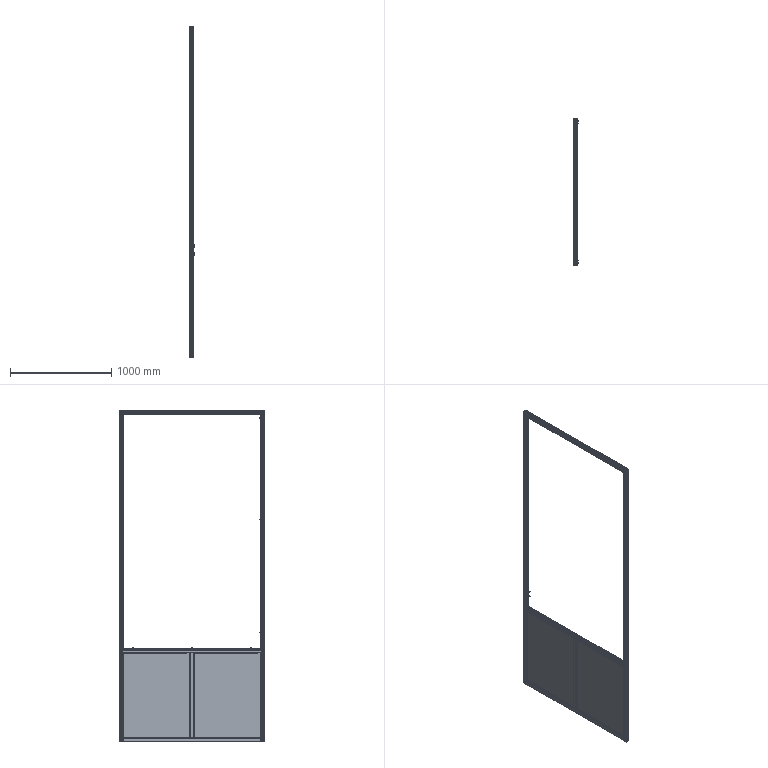Part | SolidWorks | features ReferencePattern 57, LocalLPattern 5 | 138 solids | 5490 faces | volume 13059635 mm3 | plane 3574 | cylinder 1395 | cone 475 | spline 46 | commonest cylinder face diameters 0.562 x160 8 x136 10 x104 6.8 x90 6.6 x80 2 x76